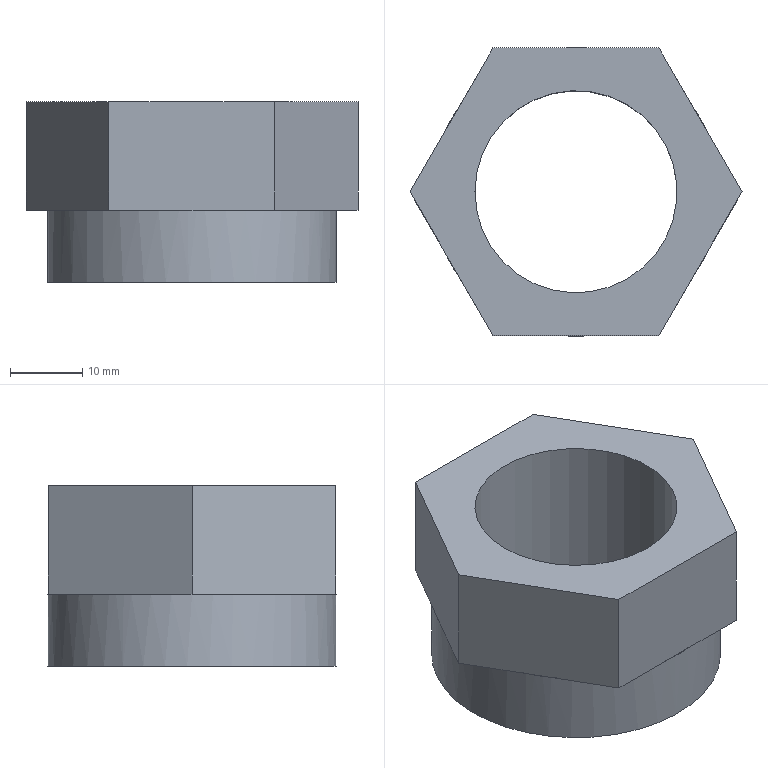Part | NX | features solid 2 | 1 solid | 22 faces | box 46 x 40 x 25 mm | volume 17788 mm3 | plane 20 | cylinder 2 | commonest cylinder face diameters 28 x1 40 x1
STEP:
#1=CARTESIAN_POINT('',(86.349,-143.479,-65.));
#2=VERTEX_POINT('',#1);
#3=CARTESIAN_POINT('',(81.5,-135.081,-65.));
#4=VERTEX_POINT('',#3);
#5=CARTESIAN_POINT('',(93.,-155.,-65.));
#6=DIRECTION('',(-0.5,0.866,0.));
#7=VECTOR('',#6,1000.);
#8=LINE('',#5,#7);
#9=EDGE_CURVE('',#2,#4,#8,.T.);
#10=ORIENTED_EDGE('',*,*,#9,.F.);
#11=CARTESIAN_POINT('',(71.803,-135.081,-65.));
#12=VERTEX_POINT('',#11);
#13=CARTESIAN_POINT('',(70.,-155.,-65.));
#14=DIRECTION('',(0.,0.,1.));
#15=DIRECTION('',(1.,0.,0.));
#16=AXIS2_PLACEMENT_3D('',#13,#14,#15);
#17=CIRCLE('',#16,20.);
#18=EDGE_CURVE('',#2,#12,#17,.T.);
#19=ORIENTED_EDGE('',*,*,#18,.T.);
#20=CARTESIAN_POINT('',(81.5,-135.081,-65.));
#21=DIRECTION('',(-1.,0.,0.));
#22=VECTOR('',#21,1000.);
#23=LINE('',#20,#22);
#24=EDGE_CURVE('',#4,#12,#23,.T.);
#25=ORIENTED_EDGE('',*,*,#24,.F.);
#26=EDGE_LOOP('',(#10,#19,#25));
#27=FACE_BOUND('',#26,.T.);
#28=CARTESIAN_POINT('',(58.5,-135.081,-65.));
#29=DIRECTION('',(0.,0.,1.));
#30=DIRECTION('',(1.,0.,0.));
#31=AXIS2_PLACEMENT_3D('',#28,#29,#30);
#32=PLANE('',#31);
#33=ADVANCED_FACE('',(#27),#32,.F.);
#34=CARTESIAN_POINT('',(68.197,-135.081,-65.));
#35=VERTEX_POINT('',#34);
#36=CARTESIAN_POINT('',(58.5,-135.081,-65.));
#37=VERTEX_POINT('',#36);
#38=CARTESIAN_POINT('',(81.5,-135.081,-65.));
#39=DIRECTION('',(-1.,0.,0.));
#40=VECTOR('',#39,1000.);
#41=LINE('',#38,#40);
#42=EDGE_CURVE('',#35,#37,#41,.T.);
#43=ORIENTED_EDGE('',*,*,#42,.F.);
#44=CARTESIAN_POINT('',(53.651,-143.479,-65.));
#45=VERTEX_POINT('',#44);
#46=CARTESIAN_POINT('',(70.,-155.,-65.));
#47=DIRECTION('',(0.,0.,1.));
#48=DIRECTION('',(1.,0.,0.));
#49=AXIS2_PLACEMENT_3D('',#46,#47,#48);
#50=CIRCLE('',#49,20.);
#51=EDGE_CURVE('',#35,#45,#50,.T.);
#52=ORIENTED_EDGE('',*,*,#51,.T.);
#53=CARTESIAN_POINT('',(58.5,-135.081,-65.));
#54=DIRECTION('',(-0.5,-0.866,0.));
#55=VECTOR('',#54,1000.);
#56=LINE('',#53,#55);
#57=EDGE_CURVE('',#37,#45,#56,.T.);
#58=ORIENTED_EDGE('',*,*,#57,.F.);
#59=EDGE_LOOP('',(#43,#52,#58));
#60=FACE_BOUND('',#59,.T.);
#61=CARTESIAN_POINT('',(58.5,-135.081,-65.));
#62=DIRECTION('',(0.,0.,1.));
#63=DIRECTION('',(1.,0.,0.));
#64=AXIS2_PLACEMENT_3D('',#61,#62,#63);
#65=PLANE('',#64);
#66=ADVANCED_FACE('',(#60),#65,.F.);
#67=CARTESIAN_POINT('',(51.849,-146.602,-65.));
#68=VERTEX_POINT('',#67);
#69=CARTESIAN_POINT('',(47.,-155.,-65.));
#70=VERTEX_POINT('',#69);
#71=CARTESIAN_POINT('',(58.5,-135.081,-65.));
#72=DIRECTION('',(-0.5,-0.866,0.));
#73=VECTOR('',#72,1000.);
#74=LINE('',#71,#73);
#75=EDGE_CURVE('',#68,#70,#74,.T.);
#76=ORIENTED_EDGE('',*,*,#75,.F.);
#77=CARTESIAN_POINT('',(51.849,-163.398,-65.));
#78=VERTEX_POINT('',#77);
#79=CARTESIAN_POINT('',(70.,-155.,-65.));
#80=DIRECTION('',(0.,0.,1.));
#81=DIRECTION('',(1.,0.,0.));
#82=AXIS2_PLACEMENT_3D('',#79,#80,#81);
#83=CIRCLE('',#82,20.);
#84=EDGE_CURVE('',#68,#78,#83,.T.);
#85=ORIENTED_EDGE('',*,*,#84,.T.);
#86=CARTESIAN_POINT('',(47.,-155.,-65.));
#87=DIRECTION('',(0.5,-0.866,0.));
#88=VECTOR('',#87,1000.);
#89=LINE('',#86,#88);
#90=EDGE_CURVE('',#70,#78,#89,.T.);
#91=ORIENTED_EDGE('',*,*,#90,.F.);
#92=EDGE_LOOP('',(#76,#85,#91));
#93=FACE_BOUND('',#92,.T.);
#94=CARTESIAN_POINT('',(58.5,-135.081,-65.));
#95=DIRECTION('',(0.,0.,1.));
#96=DIRECTION('',(1.,0.,0.));
#97=AXIS2_PLACEMENT_3D('',#94,#95,#96);
#98=PLANE('',#97);
#99=ADVANCED_FACE('',(#93),#98,.F.);
#100=CARTESIAN_POINT('',(53.651,-166.521,-65.));
#101=VERTEX_POINT('',#100);
#102=CARTESIAN_POINT('',(58.5,-174.919,-65.));
#103=VERTEX_POINT('',#102);
#104=CARTESIAN_POINT('',(47.,-155.,-65.));
#105=DIRECTION('',(0.5,-0.866,0.));
#106=VECTOR('',#105,1000.);
#107=LINE('',#104,#106);
#108=EDGE_CURVE('',#101,#103,#107,.T.);
#109=ORIENTED_EDGE('',*,*,#108,.F.);
#110=CARTESIAN_POINT('',(68.197,-174.919,-65.));
#111=VERTEX_POINT('',#110);
#112=CARTESIAN_POINT('',(70.,-155.,-65.));
#113=DIRECTION('',(0.,0.,1.));
#114=DIRECTION('',(1.,0.,0.));
#115=AXIS2_PLACEMENT_3D('',#112,#113,#114);
#116=CIRCLE('',#115,20.);
#117=EDGE_CURVE('',#101,#111,#116,.T.);
#118=ORIENTED_EDGE('',*,*,#117,.T.);
#119=CARTESIAN_POINT('',(58.5,-174.919,-65.));
#120=DIRECTION('',(1.,0.,0.));
#121=VECTOR('',#120,1000.);
#122=LINE('',#119,#121);
#123=EDGE_CURVE('',#103,#111,#122,.T.);
#124=ORIENTED_EDGE('',*,*,#123,.F.);
#125=EDGE_LOOP('',(#109,#118,#124));
#126=FACE_BOUND('',#125,.T.);
#127=CARTESIAN_POINT('',(58.5,-135.081,-65.));
#128=DIRECTION('',(0.,0.,1.));
#129=DIRECTION('',(1.,0.,0.));
#130=AXIS2_PLACEMENT_3D('',#127,#128,#129);
#131=PLANE('',#130);
#132=ADVANCED_FACE('',(#126),#131,.F.);
#133=CARTESIAN_POINT('',(71.803,-174.919,-65.));
#134=VERTEX_POINT('',#133);
#135=CARTESIAN_POINT('',(81.5,-174.919,-65.));
#136=VERTEX_POINT('',#135);
#137=CARTESIAN_POINT('',(58.5,-174.919,-65.));
#138=DIRECTION('',(1.,0.,0.));
#139=VECTOR('',#138,1000.);
#140=LINE('',#137,#139);
#141=EDGE_CURVE('',#134,#136,#140,.T.);
#142=ORIENTED_EDGE('',*,*,#141,.F.);
#143=CARTESIAN_POINT('',(86.349,-166.521,-65.));
#144=VERTEX_POINT('',#143);
#145=CARTESIAN_POINT('',(70.,-155.,-65.));
#146=DIRECTION('',(0.,0.,1.));
#147=DIRECTION('',(1.,0.,0.));
#148=AXIS2_PLACEMENT_3D('',#145,#146,#147);
#149=CIRCLE('',#148,20.);
#150=EDGE_CURVE('',#134,#144,#149,.T.);
#151=ORIENTED_EDGE('',*,*,#150,.T.);
#152=CARTESIAN_POINT('',(81.5,-174.919,-65.));
#153=DIRECTION('',(0.5,0.866,0.));
#154=VECTOR('',#153,1000.);
#155=LINE('',#152,#154);
#156=EDGE_CURVE('',#136,#144,#155,.T.);
#157=ORIENTED_EDGE('',*,*,#156,.F.);
#158=EDGE_LOOP('',(#142,#151,#157));
#159=FACE_BOUND('',#158,.T.);
#160=CARTESIAN_POINT('',(58.5,-135.081,-65.));
#161=DIRECTION('',(0.,0.,1.));
#162=DIRECTION('',(1.,0.,0.));
#163=AXIS2_PLACEMENT_3D('',#160,#161,#162);
#164=PLANE('',#163);
#165=ADVANCED_FACE('',(#159),#164,.F.);
#166=ORIENTED_EDGE('',*,*,#24,.T.);
#167=CARTESIAN_POINT('',(81.5,-135.081,-65.));
#168=DIRECTION('',(-1.,0.,0.));
#169=VECTOR('',#168,1000.);
#170=LINE('',#167,#169);
#171=EDGE_CURVE('',#12,#35,#170,.T.);
#172=ORIENTED_EDGE('',*,*,#171,.T.);
#173=ORIENTED_EDGE('',*,*,#42,.T.);
#174=CARTESIAN_POINT('',(58.5,-135.081,-50.));
#175=VERTEX_POINT('',#174);
#176=CARTESIAN_POINT('',(58.5,-135.081,-50.));
#177=DIRECTION('',(0.,0.,-1.));
#178=VECTOR('',#177,1000.);
#179=LINE('',#176,#178);
#180=EDGE_CURVE('',#175,#37,#179,.T.);
#181=ORIENTED_EDGE('',*,*,#180,.F.);
#182=CARTESIAN_POINT('',(81.5,-135.081,-50.));
#183=VERTEX_POINT('',#182);
#184=CARTESIAN_POINT('',(81.5,-135.081,-50.));
#185=DIRECTION('',(-1.,0.,0.));
#186=VECTOR('',#185,1000.);
#187=LINE('',#184,#186);
#188=EDGE_CURVE('',#183,#175,#187,.T.);
#189=ORIENTED_EDGE('',*,*,#188,.F.);
#190=CARTESIAN_POINT('',(81.5,-135.081,-50.));
#191=DIRECTION('',(0.,0.,-1.));
#192=VECTOR('',#191,1000.);
#193=LINE('',#190,#192);
#194=EDGE_CURVE('',#183,#4,#193,.T.);
#195=ORIENTED_EDGE('',*,*,#194,.T.);
#196=EDGE_LOOP('',(#166,#172,#173,#181,#189,#195));
#197=FACE_BOUND('',#196,.T.);
#198=CARTESIAN_POINT('',(81.5,-135.081,-50.));
#199=DIRECTION('',(0.,-1.,0.));
#200=DIRECTION('',(0.,0.,-1.));
#201=AXIS2_PLACEMENT_3D('',#198,#199,#200);
#202=PLANE('',#201);
#203=ADVANCED_FACE('',(#197),#202,.F.);
#204=ORIENTED_EDGE('',*,*,#57,.T.);
#205=CARTESIAN_POINT('',(58.5,-135.081,-65.));
#206=DIRECTION('',(-0.5,-0.866,0.));
#207=VECTOR('',#206,1000.);
#208=LINE('',#205,#207);
#209=EDGE_CURVE('',#45,#68,#208,.T.);
#210=ORIENTED_EDGE('',*,*,#209,.T.);
#211=ORIENTED_EDGE('',*,*,#75,.T.);
#212=CARTESIAN_POINT('',(47.,-155.,-50.));
#213=VERTEX_POINT('',#212);
#214=CARTESIAN_POINT('',(47.,-155.,-50.));
#215=DIRECTION('',(0.,0.,-1.));
#216=VECTOR('',#215,1000.);
#217=LINE('',#214,#216);
#218=EDGE_CURVE('',#213,#70,#217,.T.);
#219=ORIENTED_EDGE('',*,*,#218,.F.);
#220=CARTESIAN_POINT('',(58.5,-135.081,-50.));
#221=DIRECTION('',(-0.5,-0.866,0.));
#222=VECTOR('',#221,1000.);
#223=LINE('',#220,#222);
#224=EDGE_CURVE('',#175,#213,#223,.T.);
#225=ORIENTED_EDGE('',*,*,#224,.F.);
#226=ORIENTED_EDGE('',*,*,#180,.T.);
#227=EDGE_LOOP('',(#204,#210,#211,#219,#225,#226));
#228=FACE_BOUND('',#227,.T.);
#229=CARTESIAN_POINT('',(58.5,-135.081,-50.));
#230=DIRECTION('',(0.866,-0.5,0.));
#231=DIRECTION('',(0.5,0.866,0.));
#232=AXIS2_PLACEMENT_3D('',#229,#230,#231);
#233=PLANE('',#232);
#234=ADVANCED_FACE('',(#228),#233,.F.);
#235=ORIENTED_EDGE('',*,*,#90,.T.);
#236=CARTESIAN_POINT('',(47.,-155.,-65.));
#237=DIRECTION('',(0.5,-0.866,0.));
#238=VECTOR('',#237,1000.);
#239=LINE('',#236,#238);
#240=EDGE_CURVE('',#78,#101,#239,.T.);
#241=ORIENTED_EDGE('',*,*,#240,.T.);
#242=ORIENTED_EDGE('',*,*,#108,.T.);
#243=CARTESIAN_POINT('',(58.5,-174.919,-50.));
#244=VERTEX_POINT('',#243);
#245=CARTESIAN_POINT('',(58.5,-174.919,-50.));
#246=DIRECTION('',(0.,0.,-1.));
#247=VECTOR('',#246,1000.);
#248=LINE('',#245,#247);
#249=EDGE_CURVE('',#244,#103,#248,.T.);
#250=ORIENTED_EDGE('',*,*,#249,.F.);
#251=CARTESIAN_POINT('',(47.,-155.,-50.));
#252=DIRECTION('',(0.5,-0.866,0.));
#253=VECTOR('',#252,1000.);
#254=LINE('',#251,#253);
#255=EDGE_CURVE('',#213,#244,#254,.T.);
#256=ORIENTED_EDGE('',*,*,#255,.F.);
#257=ORIENTED_EDGE('',*,*,#218,.T.);
#258=EDGE_LOOP('',(#235,#241,#242,#250,#256,#257));
#259=FACE_BOUND('',#258,.T.);
#260=CARTESIAN_POINT('',(47.,-155.,-50.));
#261=DIRECTION('',(0.866,0.5,0.));
#262=DIRECTION('',(-0.5,0.866,0.));
#263=AXIS2_PLACEMENT_3D('',#260,#261,#262);
#264=PLANE('',#263);
#265=ADVANCED_FACE('',(#259),#264,.F.);
#266=ORIENTED_EDGE('',*,*,#123,.T.);
#267=CARTESIAN_POINT('',(58.5,-174.919,-65.));
#268=DIRECTION('',(1.,0.,0.));
#269=VECTOR('',#268,1000.);
#270=LINE('',#267,#269);
#271=EDGE_CURVE('',#111,#134,#270,.T.);
#272=ORIENTED_EDGE('',*,*,#271,.T.);
#273=ORIENTED_EDGE('',*,*,#141,.T.);
#274=CARTESIAN_POINT('',(81.5,-174.919,-50.));
#275=VERTEX_POINT('',#274);
#276=CARTESIAN_POINT('',(81.5,-174.919,-50.));
#277=DIRECTION('',(0.,0.,-1.));
#278=VECTOR('',#277,1000.);
#279=LINE('',#276,#278);
#280=EDGE_CURVE('',#275,#136,#279,.T.);
#281=ORIENTED_EDGE('',*,*,#280,.F.);
#282=CARTESIAN_POINT('',(58.5,-174.919,-50.));
#283=DIRECTION('',(1.,0.,0.));
#284=VECTOR('',#283,1000.);
#285=LINE('',#282,#284);
#286=EDGE_CURVE('',#244,#275,#285,.T.);
#287=ORIENTED_EDGE('',*,*,#286,.F.);
#288=ORIENTED_EDGE('',*,*,#249,.T.);
#289=EDGE_LOOP('',(#266,#272,#273,#281,#287,#288));
#290=FACE_BOUND('',#289,.T.);
#291=CARTESIAN_POINT('',(58.5,-174.919,-50.));
#292=DIRECTION('',(0.,1.,0.));
#293=DIRECTION('',(-1.,0.,0.));
#294=AXIS2_PLACEMENT_3D('',#291,#292,#293);
#295=PLANE('',#294);
#296=ADVANCED_FACE('',(#290),#295,.F.);
#297=ORIENTED_EDGE('',*,*,#156,.T.);
#298=CARTESIAN_POINT('',(88.151,-163.398,-65.));
#299=VERTEX_POINT('',#298);
#300=CARTESIAN_POINT('',(81.5,-174.919,-65.));
#301=DIRECTION('',(0.5,0.866,0.));
#302=VECTOR('',#301,1000.);
#303=LINE('',#300,#302);
#304=EDGE_CURVE('',#144,#299,#303,.T.);
#305=ORIENTED_EDGE('',*,*,#304,.T.);
#306=CARTESIAN_POINT('',(93.,-155.,-65.));
#307=VERTEX_POINT('',#306);
#308=CARTESIAN_POINT('',(81.5,-174.919,-65.));
#309=DIRECTION('',(0.5,0.866,0.));
#310=VECTOR('',#309,1000.);
#311=LINE('',#308,#310);
#312=EDGE_CURVE('',#299,#307,#311,.T.);
#313=ORIENTED_EDGE('',*,*,#312,.T.);
#314=CARTESIAN_POINT('',(93.,-155.,-50.));
#315=VERTEX_POINT('',#314);
#316=CARTESIAN_POINT('',(93.,-155.,-50.));
#317=DIRECTION('',(0.,0.,-1.));
#318=VECTOR('',#317,1000.);
#319=LINE('',#316,#318);
#320=EDGE_CURVE('',#315,#307,#319,.T.);
#321=ORIENTED_EDGE('',*,*,#320,.F.);
#322=CARTESIAN_POINT('',(81.5,-174.919,-50.));
#323=DIRECTION('',(0.5,0.866,0.));
#324=VECTOR('',#323,1000.);
#325=LINE('',#322,#324);
#326=EDGE_CURVE('',#275,#315,#325,.T.);
#327=ORIENTED_EDGE('',*,*,#326,.F.);
#328=ORIENTED_EDGE('',*,*,#280,.T.);
#329=EDGE_LOOP('',(#297,#305,#313,#321,#327,#328));
#330=FACE_BOUND('',#329,.T.);
#331=CARTESIAN_POINT('',(81.5,-174.919,-50.));
#332=DIRECTION('',(-0.866,0.5,0.));
#333=DIRECTION('',(-0.5,-0.866,0.));
#334=AXIS2_PLACEMENT_3D('',#331,#332,#333);
#335=PLANE('',#334);
#336=ADVANCED_FACE('',(#330),#335,.F.);
#337=CARTESIAN_POINT('',(88.151,-146.602,-65.));
#338=VERTEX_POINT('',#337);
#339=CARTESIAN_POINT('',(93.,-155.,-65.));
#340=DIRECTION('',(-0.5,0.866,0.));
#341=VECTOR('',#340,1000.);
#342=LINE('',#339,#341);
#343=EDGE_CURVE('',#307,#338,#342,.T.);
#344=ORIENTED_EDGE('',*,*,#343,.T.);
#345=CARTESIAN_POINT('',(93.,-155.,-65.));
#346=DIRECTION('',(-0.5,0.866,0.));
#347=VECTOR('',#346,1000.);
#348=LINE('',#345,#347);
#349=EDGE_CURVE('',#338,#2,#348,.T.);
#350=ORIENTED_EDGE('',*,*,#349,.T.);
#351=ORIENTED_EDGE('',*,*,#9,.T.);
#352=ORIENTED_EDGE('',*,*,#194,.F.);
#353=CARTESIAN_POINT('',(93.,-155.,-50.));
#354=DIRECTION('',(-0.5,0.866,0.));
#355=VECTOR('',#354,1000.);
#356=LINE('',#353,#355);
#357=EDGE_CURVE('',#315,#183,#356,.T.);
#358=ORIENTED_EDGE('',*,*,#357,.F.);
#359=ORIENTED_EDGE('',*,*,#320,.T.);
#360=EDGE_LOOP('',(#344,#350,#351,#352,#358,#359));
#361=FACE_BOUND('',#360,.T.);
#362=CARTESIAN_POINT('',(93.,-155.,-50.));
#363=DIRECTION('',(-0.866,-0.5,0.));
#364=DIRECTION('',(0.5,-0.866,0.));
#365=AXIS2_PLACEMENT_3D('',#362,#363,#364);
#366=PLANE('',#365);
#367=ADVANCED_FACE('',(#361),#366,.F.);
#368=CARTESIAN_POINT('',(56.,-155.,-50.));
#369=VERTEX_POINT('',#368);
#370=CARTESIAN_POINT('',(70.,-155.,-50.));
#371=DIRECTION('',(0.,0.,-1.));
#372=DIRECTION('',(-1.,0.,0.));
#373=AXIS2_PLACEMENT_3D('',#370,#371,#372);
#374=CIRCLE('',#373,14.);
#375=EDGE_CURVE('',#369,#369,#374,.T.);
#376=ORIENTED_EDGE('',*,*,#375,.F.);
#377=EDGE_LOOP('',(#376));
#378=FACE_BOUND('',#377,.T.);
#379=CARTESIAN_POINT('',(56.,-155.,-75.));
#380=VERTEX_POINT('',#379);
#381=CARTESIAN_POINT('',(70.,-155.,-75.));
#382=DIRECTION('',(0.,0.,-1.));
#383=DIRECTION('',(-1.,0.,0.));
#384=AXIS2_PLACEMENT_3D('',#381,#382,#383);
#385=CIRCLE('',#384,14.);
#386=EDGE_CURVE('',#380,#380,#385,.T.);
#387=ORIENTED_EDGE('',*,*,#386,.T.);
#388=EDGE_LOOP('',(#387));
#389=FACE_BOUND('',#388,.T.);
#390=CARTESIAN_POINT('',(70.,-155.,-50.));
#391=DIRECTION('',(0.,0.,-1.));
#392=DIRECTION('',(-1.,0.,0.));
#393=AXIS2_PLACEMENT_3D('',#390,#391,#392);
#394=CYLINDRICAL_SURFACE('',#393,14.);
#395=ADVANCED_FACE('',(#378,#389),#394,.F.);
#396=ORIENTED_EDGE('',*,*,#188,.T.);
#397=ORIENTED_EDGE('',*,*,#224,.T.);
#398=ORIENTED_EDGE('',*,*,#255,.T.);
#399=ORIENTED_EDGE('',*,*,#286,.T.);
#400=ORIENTED_EDGE('',*,*,#326,.T.);
#401=ORIENTED_EDGE('',*,*,#357,.T.);
#402=EDGE_LOOP('',(#396,#397,#398,#399,#400,#401));
#403=FACE_BOUND('',#402,.T.);
#404=ORIENTED_EDGE('',*,*,#375,.T.);
#405=EDGE_LOOP('',(#404));
#406=FACE_BOUND('',#405,.T.);
#407=CARTESIAN_POINT('',(58.5,-135.081,-50.));
#408=DIRECTION('',(0.,0.,1.));
#409=DIRECTION('',(1.,0.,0.));
#410=AXIS2_PLACEMENT_3D('',#407,#408,#409);
#411=PLANE('',#410);
#412=ADVANCED_FACE('',(#403,#406),#411,.T.);
#413=ORIENTED_EDGE('',*,*,#312,.F.);
#414=CARTESIAN_POINT('',(70.,-155.,-65.));
#415=DIRECTION('',(0.,0.,1.));
#416=DIRECTION('',(1.,0.,0.));
#417=AXIS2_PLACEMENT_3D('',#414,#415,#416);
#418=CIRCLE('',#417,20.);
#419=EDGE_CURVE('',#299,#338,#418,.T.);
#420=ORIENTED_EDGE('',*,*,#419,.T.);
#421=ORIENTED_EDGE('',*,*,#343,.F.);
#422=EDGE_LOOP('',(#413,#420,#421));
#423=FACE_BOUND('',#422,.T.);
#424=CARTESIAN_POINT('',(58.5,-135.081,-65.));
#425=DIRECTION('',(0.,0.,1.));
#426=DIRECTION('',(1.,0.,0.));
#427=AXIS2_PLACEMENT_3D('',#424,#425,#426);
#428=PLANE('',#427);
#429=ADVANCED_FACE('',(#423),#428,.F.);
#430=ORIENTED_EDGE('',*,*,#171,.F.);
#431=CARTESIAN_POINT('',(70.,-155.,-65.));
#432=DIRECTION('',(0.,0.,1.));
#433=DIRECTION('',(1.,0.,0.));
#434=AXIS2_PLACEMENT_3D('',#431,#432,#433);
#435=CIRCLE('',#434,20.);
#436=EDGE_CURVE('',#12,#35,#435,.T.);
#437=ORIENTED_EDGE('',*,*,#436,.T.);
#438=EDGE_LOOP('',(#430,#437));
#439=FACE_BOUND('',#438,.T.);
#440=CARTESIAN_POINT('',(70.,-155.,-65.));
#441=DIRECTION('',(0.,0.,1.));
#442=DIRECTION('',(1.,0.,0.));
#443=AXIS2_PLACEMENT_3D('',#440,#441,#442);
#444=PLANE('',#443);
#445=ADVANCED_FACE('',(#439),#444,.T.);
#446=ORIENTED_EDGE('',*,*,#349,.F.);
#447=CARTESIAN_POINT('',(70.,-155.,-65.));
#448=DIRECTION('',(0.,0.,1.));
#449=DIRECTION('',(1.,0.,0.));
#450=AXIS2_PLACEMENT_3D('',#447,#448,#449);
#451=CIRCLE('',#450,20.);
#452=EDGE_CURVE('',#338,#2,#451,.T.);
#453=ORIENTED_EDGE('',*,*,#452,.T.);
#454=EDGE_LOOP('',(#446,#453));
#455=FACE_BOUND('',#454,.T.);
#456=CARTESIAN_POINT('',(70.,-155.,-65.));
#457=DIRECTION('',(0.,0.,1.));
#458=DIRECTION('',(1.,0.,0.));
#459=AXIS2_PLACEMENT_3D('',#456,#457,#458);
#460=PLANE('',#459);
#461=ADVANCED_FACE('',(#455),#460,.T.);
#462=ORIENTED_EDGE('',*,*,#304,.F.);
#463=CARTESIAN_POINT('',(70.,-155.,-65.));
#464=DIRECTION('',(0.,0.,1.));
#465=DIRECTION('',(1.,0.,0.));
#466=AXIS2_PLACEMENT_3D('',#463,#464,#465);
#467=CIRCLE('',#466,20.);
#468=EDGE_CURVE('',#144,#299,#467,.T.);
#469=ORIENTED_EDGE('',*,*,#468,.T.);
#470=EDGE_LOOP('',(#462,#469));
#471=FACE_BOUND('',#470,.T.);
#472=CARTESIAN_POINT('',(70.,-155.,-65.));
#473=DIRECTION('',(0.,0.,1.));
#474=DIRECTION('',(1.,0.,0.));
#475=AXIS2_PLACEMENT_3D('',#472,#473,#474);
#476=PLANE('',#475);
#477=ADVANCED_FACE('',(#471),#476,.T.);
#478=ORIENTED_EDGE('',*,*,#271,.F.);
#479=CARTESIAN_POINT('',(70.,-155.,-65.));
#480=DIRECTION('',(0.,0.,1.));
#481=DIRECTION('',(1.,0.,0.));
#482=AXIS2_PLACEMENT_3D('',#479,#480,#481);
#483=CIRCLE('',#482,20.);
#484=EDGE_CURVE('',#111,#134,#483,.T.);
#485=ORIENTED_EDGE('',*,*,#484,.T.);
#486=EDGE_LOOP('',(#478,#485));
#487=FACE_BOUND('',#486,.T.);
#488=CARTESIAN_POINT('',(70.,-155.,-65.));
#489=DIRECTION('',(0.,0.,1.));
#490=DIRECTION('',(1.,0.,0.));
#491=AXIS2_PLACEMENT_3D('',#488,#489,#490);
#492=PLANE('',#491);
#493=ADVANCED_FACE('',(#487),#492,.T.);
#494=ORIENTED_EDGE('',*,*,#240,.F.);
#495=CARTESIAN_POINT('',(70.,-155.,-65.));
#496=DIRECTION('',(0.,0.,1.));
#497=DIRECTION('',(1.,0.,0.));
#498=AXIS2_PLACEMENT_3D('',#495,#496,#497);
#499=CIRCLE('',#498,20.);
#500=EDGE_CURVE('',#78,#101,#499,.T.);
#501=ORIENTED_EDGE('',*,*,#500,.T.);
#502=EDGE_LOOP('',(#494,#501));
#503=FACE_BOUND('',#502,.T.);
#504=CARTESIAN_POINT('',(70.,-155.,-65.));
#505=DIRECTION('',(0.,0.,1.));
#506=DIRECTION('',(1.,0.,0.));
#507=AXIS2_PLACEMENT_3D('',#504,#505,#506);
#508=PLANE('',#507);
#509=ADVANCED_FACE('',(#503),#508,.T.);
#510=ORIENTED_EDGE('',*,*,#209,.F.);
#511=CARTESIAN_POINT('',(70.,-155.,-65.));
#512=DIRECTION('',(0.,0.,1.));
#513=DIRECTION('',(1.,0.,0.));
#514=AXIS2_PLACEMENT_3D('',#511,#512,#513);
#515=CIRCLE('',#514,20.);
#516=EDGE_CURVE('',#45,#68,#515,.T.);
#517=ORIENTED_EDGE('',*,*,#516,.T.);
#518=EDGE_LOOP('',(#510,#517));
#519=FACE_BOUND('',#518,.T.);
#520=CARTESIAN_POINT('',(70.,-155.,-65.));
#521=DIRECTION('',(0.,0.,1.));
#522=DIRECTION('',(1.,0.,0.));
#523=AXIS2_PLACEMENT_3D('',#520,#521,#522);
#524=PLANE('',#523);
#525=ADVANCED_FACE('',(#519),#524,.T.);
#526=ORIENTED_EDGE('',*,*,#452,.F.);
#527=ORIENTED_EDGE('',*,*,#419,.F.);
#528=ORIENTED_EDGE('',*,*,#468,.F.);
#529=ORIENTED_EDGE('',*,*,#150,.F.);
#530=ORIENTED_EDGE('',*,*,#484,.F.);
#531=ORIENTED_EDGE('',*,*,#117,.F.);
#532=ORIENTED_EDGE('',*,*,#500,.F.);
#533=ORIENTED_EDGE('',*,*,#84,.F.);
#534=ORIENTED_EDGE('',*,*,#516,.F.);
#535=ORIENTED_EDGE('',*,*,#51,.F.);
#536=ORIENTED_EDGE('',*,*,#436,.F.);
#537=ORIENTED_EDGE('',*,*,#18,.F.);
#538=EDGE_LOOP('',(#526,#527,#528,#529,#530,#531,#532,#533,#534,#535,#536,#537));
#539=FACE_BOUND('',#538,.T.);
#540=CARTESIAN_POINT('',(90.,-155.,-75.));
#541=VERTEX_POINT('',#540);
#542=CARTESIAN_POINT('',(70.,-155.,-75.));
#543=DIRECTION('',(0.,0.,1.));
#544=DIRECTION('',(1.,0.,0.));
#545=AXIS2_PLACEMENT_3D('',#542,#543,#544);
#546=CIRCLE('',#545,20.);
#547=EDGE_CURVE('',#541,#541,#546,.T.);
#548=ORIENTED_EDGE('',*,*,#547,.T.);
#549=EDGE_LOOP('',(#548));
#550=FACE_BOUND('',#549,.T.);
#551=CARTESIAN_POINT('',(70.,-155.,-65.));
#552=DIRECTION('',(0.,0.,-1.));
#553=DIRECTION('',(-1.,0.,0.));
#554=AXIS2_PLACEMENT_3D('',#551,#552,#553);
#555=CYLINDRICAL_SURFACE('',#554,20.);
#556=ADVANCED_FACE('',(#539,#550),#555,.T.);
#557=ORIENTED_EDGE('',*,*,#547,.F.);
#558=EDGE_LOOP('',(#557));
#559=FACE_BOUND('',#558,.T.);
#560=ORIENTED_EDGE('',*,*,#386,.F.);
#561=EDGE_LOOP('',(#560));
#562=FACE_BOUND('',#561,.T.);
#563=CARTESIAN_POINT('',(70.,-155.,-75.));
#564=DIRECTION('',(0.,0.,1.));
#565=DIRECTION('',(1.,0.,0.));
#566=AXIS2_PLACEMENT_3D('',#563,#564,#565);
#567=PLANE('',#566);
#568=ADVANCED_FACE('',(#559,#562),#567,.F.);
#569=CLOSED_SHELL('',(#33,#66,#99,#132,#165,#203,#234,#265,#296,#336,#367,#395,#412,#429,#445,#461,#477,#493,#509,#525,#556,#568));
#570=MANIFOLD_SOLID_BREP('',#569);
#571=(LENGTH_UNIT()NAMED_UNIT(*)SI_UNIT(.MILLI.,.METRE.));
#572=UNCERTAINTY_MEASURE_WITH_UNIT(LENGTH_MEASURE(0.00001),#571,'','');
#573=(NAMED_UNIT(*)PLANE_ANGLE_UNIT()SI_UNIT($,.RADIAN.));
#574=(NAMED_UNIT(*)SI_UNIT($,.STERADIAN.)SOLID_ANGLE_UNIT());
#575=(GEOMETRIC_REPRESENTATION_CONTEXT(3)GLOBAL_UNCERTAINTY_ASSIGNED_CONTEXT((#572))GLOBAL_UNIT_ASSIGNED_CONTEXT((#571,#573,#574))REPRESENTATION_CONTEXT('',''));
#576=ADVANCED_BREP_SHAPE_REPRESENTATION('',(#570),#575);